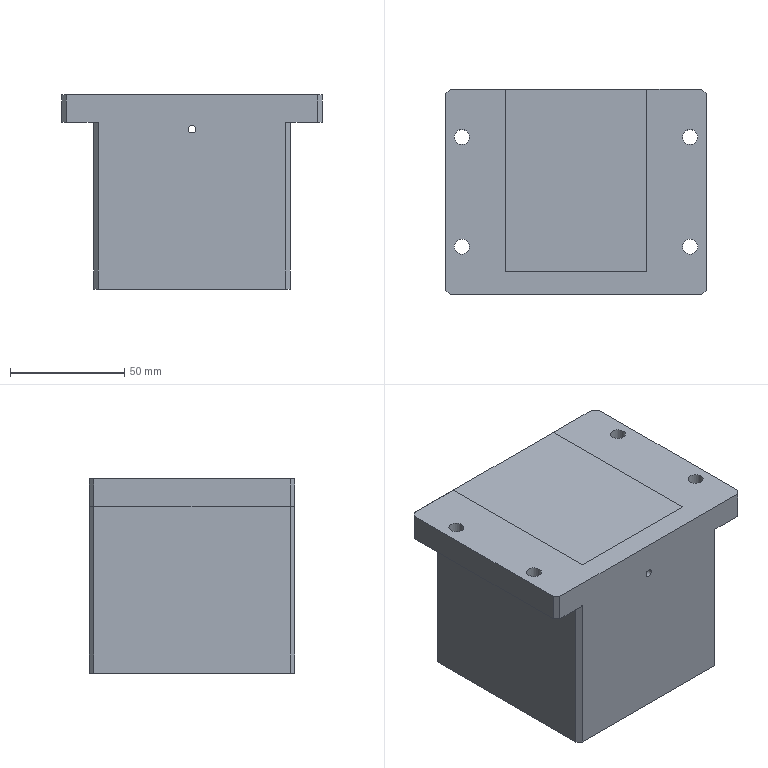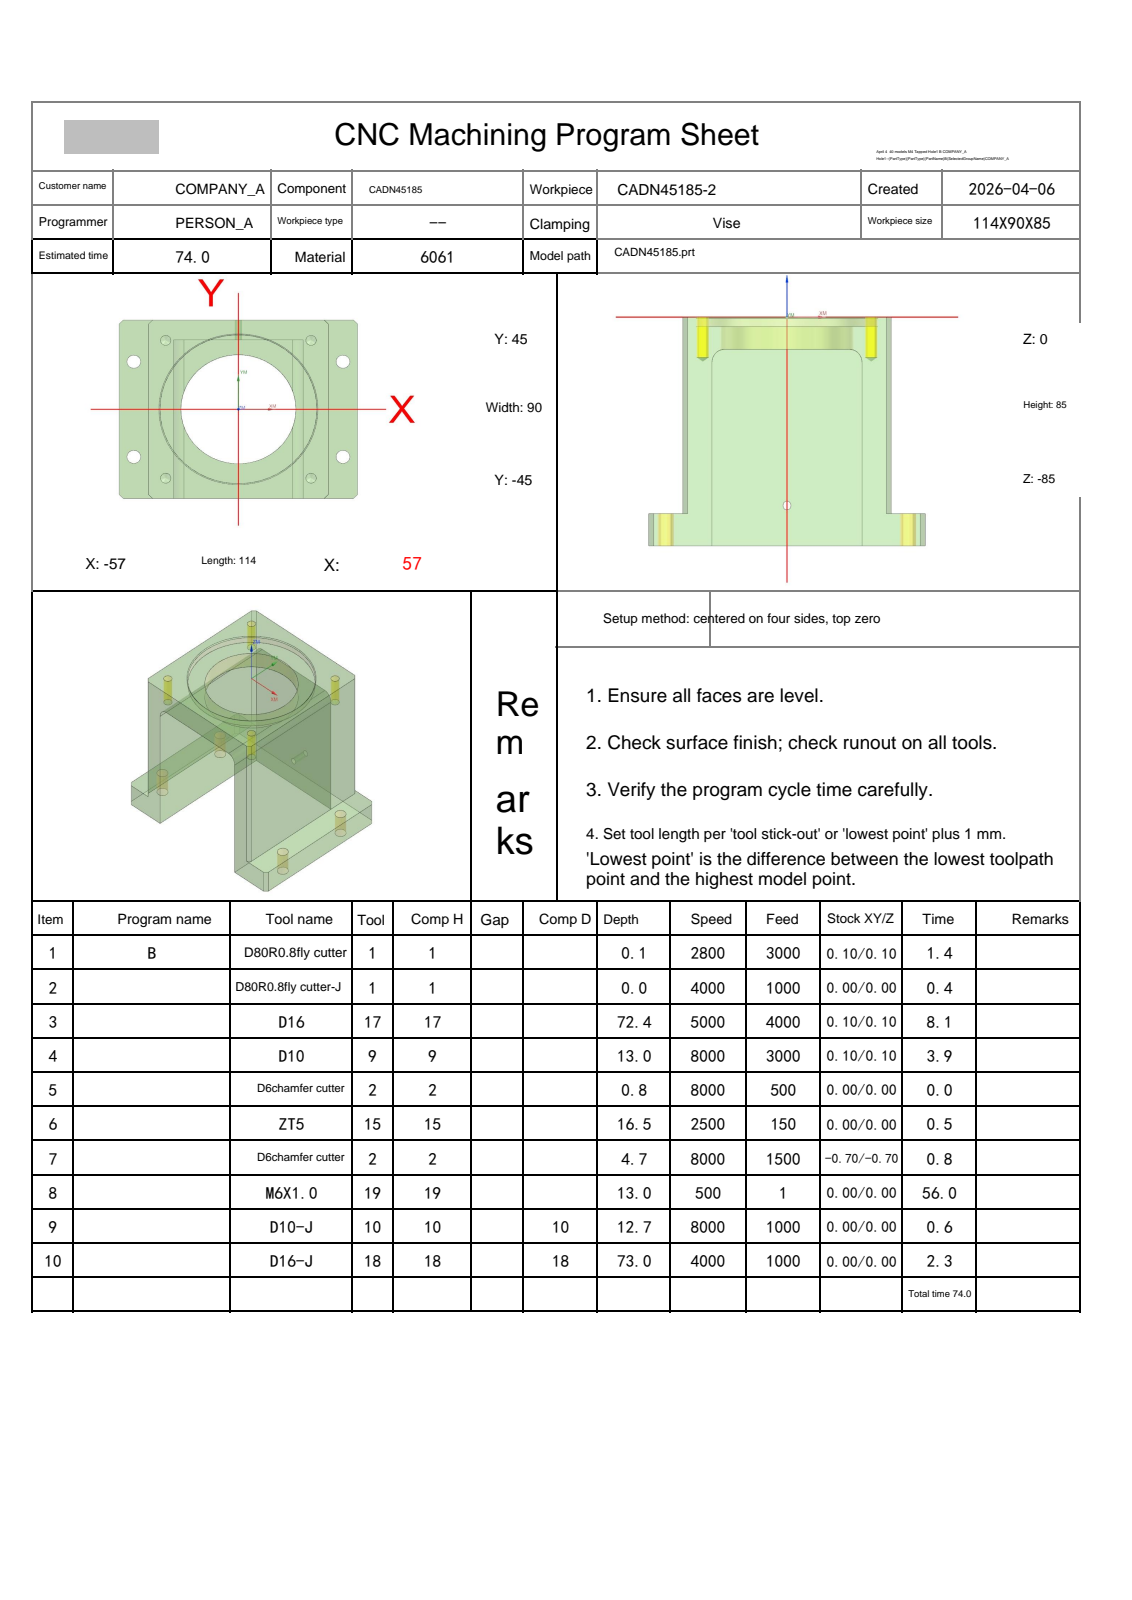NC program | NX | posted by the shop | part box 114 x 90 x 85 mm
Lines 1 to 2096 of 3620, first 1920 of 2094 lines:
%
O0001
(Machine time: 127.86 MIN)
(===Total Tool:8===)
(T1=D80R0.8飞刀 D=80.  R=0.8  D-  H01 Z=0.    )
(T17=D16    D=16.  R=0.   D-  H17 Z=-72.4 )
(T9=D10     D=10.  R=0.   D-  H09 Z=-13.  )
(T2=D6chamfer cutter   D=6.   R=0.   D-  H02 Z=-4.7  )
(T15=ZT5    D=5.   DR_a=118 D-  H15 Z=-16.5 )
(T19=M6X1.0 D=5.   DR_a=180 D-  H19 Z=-13.  )
(T10=D10-J  D=10.  R=0.   D10 H10 Z=-12.73)
(T18=D16-J  D=16.  R=0.   D18 H18 Z=-73.  )
G80 G90 G17 G49 G40
G91 G28 Z0
M01
N1 T01 M06
(D80R0.8飞刀  D=80. R=0.8 H=01 ce=0.10 di=0.10)
G00 G90 G54 X109.097 Y-21.097 M03 S2800
G43 H01 Z20.
M08
Z6.011
G01 Z4.011 F3000.
X97.097
X-89.897
G02 X-97.097 Y-13.897 I0.0 J7.2
G01 Y5.737
G02 X-89.097 Y13.737 I8. J0.0
G01 X97.097
X109.097
Z6.011
G00 Y-21.097
Z5.522
G01 Z3.522
X97.097
X-89.897
G02 X-97.097 Y-13.897 I0.0 J7.2
G01 Y5.737
G02 X-89.097 Y13.737 I8. J0.0
G01 X97.097
X109.097
Z5.522
G00 Y-21.097
Z5.033
G01 Z3.033
X97.097
X-89.897
G02 X-97.097 Y-13.897 I0.0 J7.2
G01 Y5.737
G02 X-89.097 Y13.737 I8. J0.0
G01 X97.097
X109.097
Z5.033
G00 Y-21.097
Z4.544
G01 Z2.544
X97.097
X-89.897
G02 X-97.097 Y-13.897 I0.0 J7.2
G01 Y5.737
G02 X-89.097 Y13.737 I8. J0.0
G01 X97.097
X109.097
Z4.544
G00 Y-21.097
Z4.056
G01 Z2.056
X97.097
X-89.897
G02 X-97.097 Y-13.897 I0.0 J7.2
G01 Y5.737
G02 X-89.097 Y13.737 I8. J0.0
G01 X97.097
X109.097
Z4.056
G00 Y-21.097
Z3.567
G01 Z1.567
X97.097
X-89.897
G02 X-97.097 Y-13.897 I0.0 J7.2
G01 Y5.737
G02 X-89.097 Y13.737 I8. J0.0
G01 X97.097
X109.097
Z3.567
G00 Y-21.097
Z3.078
G01 Z1.078
X97.097
X-89.897
G02 X-97.097 Y-13.897 I0.0 J7.2
G01 Y5.737
G02 X-89.097 Y13.737 I8. J0.0
G01 X97.097
X109.097
Z3.078
G00 Y-21.097
Z2.589
G01 Z.589
X97.097
X-89.897
G02 X-97.097 Y-13.897 I0.0 J7.2
G01 Y5.737
G02 X-89.097 Y13.737 I8. J0.0
G01 X97.097
X109.097
Z2.589
G00 Y-21.097
Z2.1
G01 Z.1
X97.097
X-89.897
G02 X-97.097 Y-13.897 I0.0 J7.2
G01 Y5.737
G02 X-89.097 Y13.737 I8. J0.0
G01 X97.097
X109.097
Z2.1
G00 Z20.
G91 G28 Z0.0
M05
M09
G91 G28 Z0.0
M01
N2 T01 M06
(D80R0.8飞刀-J  D=80. R=0.8 H=01 ce=0.00 di=0.00)
G00 G90 G54 X108.999 Y-20.999 M03 S4000
G43 H01 Z20.
M08
Z2.
G01 Z0.0 F1000.
X96.999
X-89.799
G02 X-96.999 Y-13.799 I0.0 J7.2
G01 Y5.639
G02 X-88.999 Y13.639 I8. J0.0
G01 X96.999
X108.999
Z2.
G00 Z20.
G91 G28 Z0.0
M05
M09
G91 G28 Z0.0
M01
N3 T17 M06
(D16  D=16. R=0. H=17 ce=0.10 di=0.10)
G00 G90 G54 X36.355 Y61.1 M03 S5000
G43 H17 Z20.
M08
Z-.598
G01 X46.728 Y50.728 F4000.
X48.728 Y48.728
G02 X51.1 Y43. I-5.728 J-5.728
G01 Y-43.
G02 X48.728 Y-48.728 I-8.1 J0.0
G01 X46.728 Y-50.728
X36.355 Y-61.1
G00 Z-1.197
G01 X46.728 Y-50.728
X48.728 Y-48.728
G03 X51.1 Y-43. I-5.728 J5.728
G01 Y43.
G03 X48.728 Y48.728 I-8.1 J0.0
G01 X46.728 Y50.728
X36.355 Y61.1
G00 Z-1.795
G01 X46.728 Y50.728
X48.728 Y48.728
G02 X51.1 Y43. I-5.728 J-5.728
G01 Y-43.
G02 X48.728 Y-48.728 I-8.1 J0.0
G01 X46.728 Y-50.728
X36.355 Y-61.1
G00 Z-2.393
G01 X46.728 Y-50.728
X48.728 Y-48.728
G03 X51.1 Y-43. I-5.728 J5.728
G01 Y43.
G03 X48.728 Y48.728 I-8.1 J0.0
G01 X46.728 Y50.728
X36.355 Y61.1
G00 Z-2.992
G01 X46.728 Y50.728
X48.728 Y48.728
G02 X51.1 Y43. I-5.728 J-5.728
G01 Y-43.
G02 X48.728 Y-48.728 I-8.1 J0.0
G01 X46.728 Y-50.728
X36.355 Y-61.1
G00 Z-3.59
G01 X46.728 Y-50.728
X48.728 Y-48.728
G03 X51.1 Y-43. I-5.728 J5.728
G01 Y43.
G03 X48.728 Y48.728 I-8.1 J0.0
G01 X46.728 Y50.728
X36.355 Y61.1
G00 Z-4.189
G01 X46.728 Y50.728
X48.728 Y48.728
G02 X51.1 Y43. I-5.728 J-5.728
G01 Y-43.
G02 X48.728 Y-48.728 I-8.1 J0.0
G01 X46.728 Y-50.728
X36.355 Y-61.1
G00 Z-4.787
G01 X46.728 Y-50.728
X48.728 Y-48.728
G03 X51.1 Y-43. I-5.728 J5.728
G01 Y43.
G03 X48.728 Y48.728 I-8.1 J0.0
G01 X46.728 Y50.728
X36.355 Y61.1
G00 Z-5.385
G01 X46.728 Y50.728
X48.728 Y48.728
G02 X51.1 Y43. I-5.728 J-5.728
G01 Y-43.
G02 X48.728 Y-48.728 I-8.1 J0.0
G01 X46.728 Y-50.728
X36.355 Y-61.1
G00 Z-5.984
G01 X46.728 Y-50.728
X48.728 Y-48.728
G03 X51.1 Y-43. I-5.728 J5.728
G01 Y43.
G03 X48.728 Y48.728 I-8.1 J0.0
G01 X46.728 Y50.728
X36.355 Y61.1
G00 Z-6.582
G01 X46.728 Y50.728
X48.728 Y48.728
G02 X51.1 Y43. I-5.728 J-5.728
G01 Y-43.
G02 X48.728 Y-48.728 I-8.1 J0.0
G01 X46.728 Y-50.728
X36.355 Y-61.1
G00 Z-7.18
G01 X46.728 Y-50.728
X48.728 Y-48.728
G03 X51.1 Y-43. I-5.728 J5.728
G01 Y43.
G03 X48.728 Y48.728 I-8.1 J0.0
G01 X46.728 Y50.728
X36.355 Y61.1
G00 Z-7.779
G01 X46.728 Y50.728
X48.728 Y48.728
G02 X51.1 Y43. I-5.728 J-5.728
G01 Y-43.
G02 X48.728 Y-48.728 I-8.1 J0.0
G01 X46.728 Y-50.728
X36.355 Y-61.1
G00 Z-8.377
G01 X46.728 Y-50.728
X48.728 Y-48.728
G03 X51.1 Y-43. I-5.728 J5.728
G01 Y43.
G03 X48.728 Y48.728 I-8.1 J0.0
G01 X46.728 Y50.728
X36.355 Y61.1
G00 Z-8.975
G01 X46.728 Y50.728
X48.728 Y48.728
G02 X51.1 Y43. I-5.728 J-5.728
G01 Y-43.
G02 X48.728 Y-48.728 I-8.1 J0.0
G01 X46.728 Y-50.728
X36.355 Y-61.1
G00 Z-9.574
G01 X46.728 Y-50.728
X48.728 Y-48.728
G03 X51.1 Y-43. I-5.728 J5.728
G01 Y43.
G03 X48.728 Y48.728 I-8.1 J0.0
G01 X46.728 Y50.728
X36.355 Y61.1
G00 Z-10.172
G01 X46.728 Y50.728
X48.728 Y48.728
G02 X51.1 Y43. I-5.728 J-5.728
G01 Y-43.
G02 X48.728 Y-48.728 I-8.1 J0.0
G01 X46.728 Y-50.728
X36.355 Y-61.1
G00 Z-10.77
G01 X46.728 Y-50.728
X48.728 Y-48.728
G03 X51.1 Y-43. I-5.728 J5.728
G01 Y43.
G03 X48.728 Y48.728 I-8.1 J0.0
G01 X46.728 Y50.728
X36.355 Y61.1
G00 Z-11.369
G01 X46.728 Y50.728
X48.728 Y48.728
G02 X51.1 Y43. I-5.728 J-5.728
G01 Y-43.
G02 X48.728 Y-48.728 I-8.1 J0.0
G01 X46.728 Y-50.728
X36.355 Y-61.1
G00 Z-11.967
G01 X46.728 Y-50.728
X48.728 Y-48.728
G03 X51.1 Y-43. I-5.728 J5.728
G01 Y43.
G03 X48.728 Y48.728 I-8.1 J0.0
G01 X46.728 Y50.728
X36.355 Y61.1
G00 Z-12.566
G01 X46.728 Y50.728
X48.728 Y48.728
G02 X51.1 Y43. I-5.728 J-5.728
G01 Y-43.
G02 X48.728 Y-48.728 I-8.1 J0.0
G01 X46.728 Y-50.728
X36.355 Y-61.1
G00 Z-13.164
G01 X46.728 Y-50.728
X48.728 Y-48.728
G03 X51.1 Y-43. I-5.728 J5.728
G01 Y43.
G03 X48.728 Y48.728 I-8.1 J0.0
G01 X46.728 Y50.728
X36.355 Y61.1
G00 Z-13.762
G01 X46.728 Y50.728
X48.728 Y48.728
G02 X51.1 Y43. I-5.728 J-5.728
G01 Y-43.
G02 X48.728 Y-48.728 I-8.1 J0.0
G01 X46.728 Y-50.728
X36.355 Y-61.1
G00 Z-14.361
G01 X46.728 Y-50.728
X48.728 Y-48.728
G03 X51.1 Y-43. I-5.728 J5.728
G01 Y43.
G03 X48.728 Y48.728 I-8.1 J0.0
G01 X46.728 Y50.728
X36.355 Y61.1
G00 Z-14.959
G01 X46.728 Y50.728
X48.728 Y48.728
G02 X51.1 Y43. I-5.728 J-5.728
G01 Y-43.
G02 X48.728 Y-48.728 I-8.1 J0.0
G01 X46.728 Y-50.728
X36.355 Y-61.1
G00 Z-15.557
G01 X46.728 Y-50.728
X48.728 Y-48.728
G03 X51.1 Y-43. I-5.728 J5.728
G01 Y43.
G03 X48.728 Y48.728 I-8.1 J0.0
G01 X46.728 Y50.728
X36.355 Y61.1
G00 Z-16.156
G01 X46.728 Y50.728
X48.728 Y48.728
G02 X51.1 Y43. I-5.728 J-5.728
G01 Y-43.
G02 X48.728 Y-48.728 I-8.1 J0.0
G01 X46.728 Y-50.728
X36.355 Y-61.1
G00 Z-16.754
G01 X46.728 Y-50.728
X48.728 Y-48.728
G03 X51.1 Y-43. I-5.728 J5.728
G01 Y43.
G03 X48.728 Y48.728 I-8.1 J0.0
G01 X46.728 Y50.728
X36.355 Y61.1
G00 Z-17.352
G01 X46.728 Y50.728
X48.728 Y48.728
G02 X51.1 Y43. I-5.728 J-5.728
G01 Y-43.
G02 X48.728 Y-48.728 I-8.1 J0.0
G01 X46.728 Y-50.728
X36.355 Y-61.1
G00 Z-17.951
G01 X46.728 Y-50.728
X48.728 Y-48.728
G03 X51.1 Y-43. I-5.728 J5.728
G01 Y43.
G03 X48.728 Y48.728 I-8.1 J0.0
G01 X46.728 Y50.728
X36.355 Y61.1
G00 Z-18.549
G01 X46.728 Y50.728
X48.728 Y48.728
G02 X51.1 Y43. I-5.728 J-5.728
G01 Y-43.
G02 X48.728 Y-48.728 I-8.1 J0.0
G01 X46.728 Y-50.728
X36.355 Y-61.1
G00 Z-19.148
G01 X46.728 Y-50.728
X48.728 Y-48.728
G03 X51.1 Y-43. I-5.728 J5.728
G01 Y43.
G03 X48.728 Y48.728 I-8.1 J0.0
G01 X46.728 Y50.728
X36.355 Y61.1
G00 Z-19.746
G01 X46.728 Y50.728
X48.728 Y48.728
G02 X51.1 Y43. I-5.728 J-5.728
G01 Y-43.
G02 X48.728 Y-48.728 I-8.1 J0.0
G01 X46.728 Y-50.728
X36.355 Y-61.1
G00 Z-20.344
G01 X46.728 Y-50.728
X48.728 Y-48.728
G03 X51.1 Y-43. I-5.728 J5.728
G01 Y43.
G03 X48.728 Y48.728 I-8.1 J0.0
G01 X46.728 Y50.728
X36.355 Y61.1
G00 Z-20.943
G01 X46.728 Y50.728
X48.728 Y48.728
G02 X51.1 Y43. I-5.728 J-5.728
G01 Y-43.
G02 X48.728 Y-48.728 I-8.1 J0.0
G01 X46.728 Y-50.728
X36.355 Y-61.1
G00 Z-21.541
G01 X46.728 Y-50.728
X48.728 Y-48.728
G03 X51.1 Y-43. I-5.728 J5.728
G01 Y43.
G03 X48.728 Y48.728 I-8.1 J0.0
G01 X46.728 Y50.728
X36.355 Y61.1
G00 Z-22.139
G01 X46.728 Y50.728
X48.728 Y48.728
G02 X51.1 Y43. I-5.728 J-5.728
G01 Y-43.
G02 X48.728 Y-48.728 I-8.1 J0.0
G01 X46.728 Y-50.728
X36.355 Y-61.1
G00 Z-22.738
G01 X46.728 Y-50.728
X48.728 Y-48.728
G03 X51.1 Y-43. I-5.728 J5.728
G01 Y43.
G03 X48.728 Y48.728 I-8.1 J0.0
G01 X46.728 Y50.728
X36.355 Y61.1
G00 Z-23.336
G01 X46.728 Y50.728
X48.728 Y48.728
G02 X51.1 Y43. I-5.728 J-5.728
G01 Y-43.
G02 X48.728 Y-48.728 I-8.1 J0.0
G01 X46.728 Y-50.728
X36.355 Y-61.1
G00 Z-23.934
G01 X46.728 Y-50.728
X48.728 Y-48.728
G03 X51.1 Y-43. I-5.728 J5.728
G01 Y43.
G03 X48.728 Y48.728 I-8.1 J0.0
G01 X46.728 Y50.728
X36.355 Y61.1
G00 Z-24.533
G01 X46.728 Y50.728
X48.728 Y48.728
G02 X51.1 Y43. I-5.728 J-5.728
G01 Y-43.
G02 X48.728 Y-48.728 I-8.1 J0.0
G01 X46.728 Y-50.728
X36.355 Y-61.1
G00 Z-25.131
G01 X46.728 Y-50.728
X48.728 Y-48.728
G03 X51.1 Y-43. I-5.728 J5.728
G01 Y43.
G03 X48.728 Y48.728 I-8.1 J0.0
G01 X46.728 Y50.728
X36.355 Y61.1
G00 Z-25.73
G01 X46.728 Y50.728
X48.728 Y48.728
G02 X51.1 Y43. I-5.728 J-5.728
G01 Y-43.
G02 X48.728 Y-48.728 I-8.1 J0.0
G01 X46.728 Y-50.728
X36.355 Y-61.1
G00 Z-26.328
G01 X46.728 Y-50.728
X48.728 Y-48.728
G03 X51.1 Y-43. I-5.728 J5.728
G01 Y43.
G03 X48.728 Y48.728 I-8.1 J0.0
G01 X46.728 Y50.728
X36.355 Y61.1
G00 Z-26.926
G01 X46.728 Y50.728
X48.728 Y48.728
G02 X51.1 Y43. I-5.728 J-5.728
G01 Y-43.
G02 X48.728 Y-48.728 I-8.1 J0.0
G01 X46.728 Y-50.728
X36.355 Y-61.1
G00 Z-27.525
G01 X46.728 Y-50.728
X48.728 Y-48.728
G03 X51.1 Y-43. I-5.728 J5.728
G01 Y43.
G03 X48.728 Y48.728 I-8.1 J0.0
G01 X46.728 Y50.728
X36.355 Y61.1
G00 Z-28.123
G01 X46.728 Y50.728
X48.728 Y48.728
G02 X51.1 Y43. I-5.728 J-5.728
G01 Y-43.
G02 X48.728 Y-48.728 I-8.1 J0.0
G01 X46.728 Y-50.728
X36.355 Y-61.1
G00 Z-28.721
G01 X46.728 Y-50.728
X48.728 Y-48.728
G03 X51.1 Y-43. I-5.728 J5.728
G01 Y43.
G03 X48.728 Y48.728 I-8.1 J0.0
G01 X46.728 Y50.728
X36.355 Y61.1
G00 Z-29.32
G01 X46.728 Y50.728
X48.728 Y48.728
G02 X51.1 Y43. I-5.728 J-5.728
G01 Y-43.
G02 X48.728 Y-48.728 I-8.1 J0.0
G01 X46.728 Y-50.728
X36.355 Y-61.1
G00 Z-29.918
G01 X46.728 Y-50.728
X48.728 Y-48.728
G03 X51.1 Y-43. I-5.728 J5.728
G01 Y43.
G03 X48.728 Y48.728 I-8.1 J0.0
G01 X46.728 Y50.728
X36.355 Y61.1
G00 Z-30.516
G01 X46.728 Y50.728
X48.728 Y48.728
G02 X51.1 Y43. I-5.728 J-5.728
G01 Y-43.
G02 X48.728 Y-48.728 I-8.1 J0.0
G01 X46.728 Y-50.728
X36.355 Y-61.1
G00 Z-31.115
G01 X46.728 Y-50.728
X48.728 Y-48.728
G03 X51.1 Y-43. I-5.728 J5.728
G01 Y43.
G03 X48.728 Y48.728 I-8.1 J0.0
G01 X46.728 Y50.728
X36.355 Y61.1
G00 Z-31.713
G01 X46.728 Y50.728
X48.728 Y48.728
G02 X51.1 Y43. I-5.728 J-5.728
G01 Y-43.
G02 X48.728 Y-48.728 I-8.1 J0.0
G01 X46.728 Y-50.728
X36.355 Y-61.1
G00 Z-32.311
G01 X46.728 Y-50.728
X48.728 Y-48.728
G03 X51.1 Y-43. I-5.728 J5.728
G01 Y43.
G03 X48.728 Y48.728 I-8.1 J0.0
G01 X46.728 Y50.728
X36.355 Y61.1
G00 Z-32.91
G01 X46.728 Y50.728
X48.728 Y48.728
G02 X51.1 Y43. I-5.728 J-5.728
G01 Y-43.
G02 X48.728 Y-48.728 I-8.1 J0.0
G01 X46.728 Y-50.728
X36.355 Y-61.1
G00 Z-33.508
G01 X46.728 Y-50.728
X48.728 Y-48.728
G03 X51.1 Y-43. I-5.728 J5.728
G01 Y43.
G03 X48.728 Y48.728 I-8.1 J0.0
G01 X46.728 Y50.728
X36.355 Y61.1
G00 Z-34.107
G01 X46.728 Y50.728
X48.728 Y48.728
G02 X51.1 Y43. I-5.728 J-5.728
G01 Y-43.
G02 X48.728 Y-48.728 I-8.1 J0.0
G01 X46.728 Y-50.728
X36.355 Y-61.1
G00 Z-34.705
G01 X46.728 Y-50.728
X48.728 Y-48.728
G03 X51.1 Y-43. I-5.728 J5.728
G01 Y43.
G03 X48.728 Y48.728 I-8.1 J0.0
G01 X46.728 Y50.728
X36.355 Y61.1
G00 Z-35.303
G01 X46.728 Y50.728
X48.728 Y48.728
G02 X51.1 Y43. I-5.728 J-5.728
G01 Y-43.
G02 X48.728 Y-48.728 I-8.1 J0.0
G01 X46.728 Y-50.728
X36.355 Y-61.1
G00 Z-35.902
G01 X46.728 Y-50.728
X48.728 Y-48.728
G03 X51.1 Y-43. I-5.728 J5.728
G01 Y43.
G03 X48.728 Y48.728 I-8.1 J0.0
G01 X46.728 Y50.728
X36.355 Y61.1
G00 Z-36.5
G01 X46.728 Y50.728
X48.728 Y48.728
G02 X51.1 Y43. I-5.728 J-5.728
G01 Y-43.
G02 X48.728 Y-48.728 I-8.1 J0.0
G01 X46.728 Y-50.728
X36.355 Y-61.1
G00 Z-37.098
G01 X46.728 Y-50.728
X48.728 Y-48.728
G03 X51.1 Y-43. I-5.728 J5.728
G01 Y43.
G03 X48.728 Y48.728 I-8.1 J0.0
G01 X46.728 Y50.728
X36.355 Y61.1
G00 Z-37.697
G01 X46.728 Y50.728
X48.728 Y48.728
G02 X51.1 Y43. I-5.728 J-5.728
G01 Y-43.
G02 X48.728 Y-48.728 I-8.1 J0.0
G01 X46.728 Y-50.728
X36.355 Y-61.1
G00 Z-38.295
G01 X46.728 Y-50.728
X48.728 Y-48.728
G03 X51.1 Y-43. I-5.728 J5.728
G01 Y43.
G03 X48.728 Y48.728 I-8.1 J0.0
G01 X46.728 Y50.728
X36.355 Y61.1
G00 Z-38.893
G01 X46.728 Y50.728
X48.728 Y48.728
G02 X51.1 Y43. I-5.728 J-5.728
G01 Y-43.
G02 X48.728 Y-48.728 I-8.1 J0.0
G01 X46.728 Y-50.728
X36.355 Y-61.1
G00 Z-39.492
G01 X46.728 Y-50.728
X48.728 Y-48.728
G03 X51.1 Y-43. I-5.728 J5.728
G01 Y43.
G03 X48.728 Y48.728 I-8.1 J0.0
G01 X46.728 Y50.728
X36.355 Y61.1
G00 Z-40.09
G01 X46.728 Y50.728
X48.728 Y48.728
G02 X51.1 Y43. I-5.728 J-5.728
G01 Y-43.
G02 X48.728 Y-48.728 I-8.1 J0.0
G01 X46.728 Y-50.728
X36.355 Y-61.1
G00 Z-40.689
G01 X46.728 Y-50.728
X48.728 Y-48.728
G03 X51.1 Y-43. I-5.728 J5.728
G01 Y43.
G03 X48.728 Y48.728 I-8.1 J0.0
G01 X46.728 Y50.728
X36.355 Y61.1
G00 Z-41.287
G01 X46.728 Y50.728
X48.728 Y48.728
G02 X51.1 Y43. I-5.728 J-5.728
G01 Y-43.
G02 X48.728 Y-48.728 I-8.1 J0.0
G01 X46.728 Y-50.728
X36.355 Y-61.1
G00 Z-41.885
G01 X46.728 Y-50.728
X48.728 Y-48.728
G03 X51.1 Y-43. I-5.728 J5.728
G01 Y43.
G03 X48.728 Y48.728 I-8.1 J0.0
G01 X46.728 Y50.728
X36.355 Y61.1
G00 Z-42.484
G01 X46.728 Y50.728
X48.728 Y48.728
G02 X51.1 Y43. I-5.728 J-5.728
G01 Y-43.
G02 X48.728 Y-48.728 I-8.1 J0.0
G01 X46.728 Y-50.728
X36.355 Y-61.1
G00 Z-43.082
G01 X46.728 Y-50.728
X48.728 Y-48.728
G03 X51.1 Y-43. I-5.728 J5.728
G01 Y43.
G03 X48.728 Y48.728 I-8.1 J0.0
G01 X46.728 Y50.728
X36.355 Y61.1
G00 Z-43.68
G01 X46.728 Y50.728
X48.728 Y48.728
G02 X51.1 Y43. I-5.728 J-5.728
G01 Y-43.
G02 X48.728 Y-48.728 I-8.1 J0.0
G01 X46.728 Y-50.728
X36.355 Y-61.1
G00 Z-44.279
G01 X46.728 Y-50.728
X48.728 Y-48.728
G03 X51.1 Y-43. I-5.728 J5.728
G01 Y43.
G03 X48.728 Y48.728 I-8.1 J0.0
G01 X46.728 Y50.728
X36.355 Y61.1
G00 Z-44.877
G01 X46.728 Y50.728
X48.728 Y48.728
G02 X51.1 Y43. I-5.728 J-5.728
G01 Y-43.
G02 X48.728 Y-48.728 I-8.1 J0.0
G01 X46.728 Y-50.728
X36.355 Y-61.1
G00 Z-45.475
G01 X46.728 Y-50.728
X48.728 Y-48.728
G03 X51.1 Y-43. I-5.728 J5.728
G01 Y43.
G03 X48.728 Y48.728 I-8.1 J0.0
G01 X46.728 Y50.728
X36.355 Y61.1
G00 Z-46.074
G01 X46.728 Y50.728
X48.728 Y48.728
G02 X51.1 Y43. I-5.728 J-5.728
G01 Y-43.
G02 X48.728 Y-48.728 I-8.1 J0.0
G01 X46.728 Y-50.728
X36.355 Y-61.1
G00 Z-46.672
G01 X46.728 Y-50.728
X48.728 Y-48.728
G03 X51.1 Y-43. I-5.728 J5.728
G01 Y43.
G03 X48.728 Y48.728 I-8.1 J0.0
G01 X46.728 Y50.728
X36.355 Y61.1
G00 Z-47.27
G01 X46.728 Y50.728
X48.728 Y48.728
G02 X51.1 Y43. I-5.728 J-5.728
G01 Y-43.
G02 X48.728 Y-48.728 I-8.1 J0.0
G01 X46.728 Y-50.728
X36.355 Y-61.1
G00 Z-47.869
G01 X46.728 Y-50.728
X48.728 Y-48.728
G03 X51.1 Y-43. I-5.728 J5.728
G01 Y43.
G03 X48.728 Y48.728 I-8.1 J0.0
G01 X46.728 Y50.728
X36.355 Y61.1
G00 Z-48.467
G01 X46.728 Y50.728
X48.728 Y48.728
G02 X51.1 Y43. I-5.728 J-5.728
G01 Y-43.
G02 X48.728 Y-48.728 I-8.1 J0.0
G01 X46.728 Y-50.728
X36.355 Y-61.1
G00 Z-49.066
G01 X46.728 Y-50.728
X48.728 Y-48.728
G03 X51.1 Y-43. I-5.728 J5.728
G01 Y43.
G03 X48.728 Y48.728 I-8.1 J0.0
G01 X46.728 Y50.728
X36.355 Y61.1
G00 Z-49.664
G01 X46.728 Y50.728
X48.728 Y48.728
G02 X51.1 Y43. I-5.728 J-5.728
G01 Y-43.
G02 X48.728 Y-48.728 I-8.1 J0.0
G01 X46.728 Y-50.728
X36.355 Y-61.1
G00 Z-50.262
G01 X46.728 Y-50.728
X48.728 Y-48.728
G03 X51.1 Y-43. I-5.728 J5.728
G01 Y43.
G03 X48.728 Y48.728 I-8.1 J0.0
G01 X46.728 Y50.728
X36.355 Y61.1
G00 Z-50.861
G01 X46.728 Y50.728
X48.728 Y48.728
G02 X51.1 Y43. I-5.728 J-5.728
G01 Y-43.
G02 X48.728 Y-48.728 I-8.1 J0.0
G01 X46.728 Y-50.728
X36.355 Y-61.1
G00 Z-51.459
G01 X46.728 Y-50.728
X48.728 Y-48.728
G03 X51.1 Y-43. I-5.728 J5.728
G01 Y43.
G03 X48.728 Y48.728 I-8.1 J0.0
G01 X46.728 Y50.728
X36.355 Y61.1
G00 Z-52.057
G01 X46.728 Y50.728
X48.728 Y48.728
G02 X51.1 Y43. I-5.728 J-5.728
G01 Y-43.
G02 X48.728 Y-48.728 I-8.1 J0.0
G01 X46.728 Y-50.728
X36.355 Y-61.1
G00 Z-52.656
G01 X46.728 Y-50.728
X48.728 Y-48.728
G03 X51.1 Y-43. I-5.728 J5.728
G01 Y43.
G03 X48.728 Y48.728 I-8.1 J0.0
G01 X46.728 Y50.728
X36.355 Y61.1
G00 Z-53.254
G01 X46.728 Y50.728
X48.728 Y48.728
G02 X51.1 Y43. I-5.728 J-5.728
G01 Y-43.
G02 X48.728 Y-48.728 I-8.1 J0.0
G01 X46.728 Y-50.728
X36.355 Y-61.1
G00 Z-53.852
G01 X46.728 Y-50.728
X48.728 Y-48.728
G03 X51.1 Y-43. I-5.728 J5.728
G01 Y43.
G03 X48.728 Y48.728 I-8.1 J0.0
G01 X46.728 Y50.728
X36.355 Y61.1
G00 Z-54.451
G01 X46.728 Y50.728
X48.728 Y48.728
G02 X51.1 Y43. I-5.728 J-5.728
G01 Y-43.
G02 X48.728 Y-48.728 I-8.1 J0.0
G01 X46.728 Y-50.728
X36.355 Y-61.1
G00 Z-55.049
G01 X46.728 Y-50.728
X48.728 Y-48.728
G03 X51.1 Y-43. I-5.728 J5.728
G01 Y43.
G03 X48.728 Y48.728 I-8.1 J0.0
G01 X46.728 Y50.728
X36.355 Y61.1
G00 Z-55.648
G01 X46.728 Y50.728
X48.728 Y48.728
G02 X51.1 Y43. I-5.728 J-5.728
G01 Y-43.
G02 X48.728 Y-48.728 I-8.1 J0.0
G01 X46.728 Y-50.728
X36.355 Y-61.1
G00 Z-56.246
G01 X46.728 Y-50.728
X48.728 Y-48.728
G03 X51.1 Y-43. I-5.728 J5.728
G01 Y43.
G03 X48.728 Y48.728 I-8.1 J0.0
G01 X46.728 Y50.728
X36.355 Y61.1
G00 Z-56.844
G01 X46.728 Y50.728
X48.728 Y48.728
G02 X51.1 Y43. I-5.728 J-5.728
G01 Y-43.
G02 X48.728 Y-48.728 I-8.1 J0.0
G01 X46.728 Y-50.728
X36.355 Y-61.1
G00 Z-57.443
G01 X46.728 Y-50.728
X48.728 Y-48.728
G03 X51.1 Y-43. I-5.728 J5.728
G01 Y43.
G03 X48.728 Y48.728 I-8.1 J0.0
G01 X46.728 Y50.728
X36.355 Y61.1
G00 Z-58.041
G01 X46.728 Y50.728
X48.728 Y48.728
G02 X51.1 Y43. I-5.728 J-5.728
G01 Y-43.
G02 X48.728 Y-48.728 I-8.1 J0.0
G01 X46.728 Y-50.728
X36.355 Y-61.1
G00 Z-58.639
G01 X46.728 Y-50.728
X48.728 Y-48.728
G03 X51.1 Y-43. I-5.728 J5.728
G01 Y43.
G03 X48.728 Y48.728 I-8.1 J0.0
G01 X46.728 Y50.728
X36.355 Y61.1
G00 Z-59.238
G01 X46.728 Y50.728
X48.728 Y48.728
G02 X51.1 Y43. I-5.728 J-5.728
G01 Y-43.
G02 X48.728 Y-48.728 I-8.1 J0.0
G01 X46.728 Y-50.728
X36.355 Y-61.1
G00 Z-59.836
G01 X46.728 Y-50.728
X48.728 Y-48.728
G03 X51.1 Y-43. I-5.728 J5.728
G01 Y43.
G03 X48.728 Y48.728 I-8.1 J0.0
G01 X46.728 Y50.728
X36.355 Y61.1
G00 Z-60.434
G01 X46.728 Y50.728
X48.728 Y48.728
G02 X51.1 Y43. I-5.728 J-5.728
G01 Y-43.
G02 X48.728 Y-48.728 I-8.1 J0.0
G01 X46.728 Y-50.728
X36.355 Y-61.1
G00 Z-61.033
G01 X46.728 Y-50.728
X48.728 Y-48.728
G03 X51.1 Y-43. I-5.728 J5.728
G01 Y43.
G03 X48.728 Y48.728 I-8.1 J0.0
G01 X46.728 Y50.728
X36.355 Y61.1
G00 Z-61.631
G01 X46.728 Y50.728
X48.728 Y48.728
G02 X51.1 Y43. I-5.728 J-5.728
G01 Y-43.
G02 X48.728 Y-48.728 I-8.1 J0.0
G01 X46.728 Y-50.728
X36.355 Y-61.1
G00 Z-62.23
G01 X46.728 Y-50.728
X48.728 Y-48.728
G03 X51.1 Y-43. I-5.728 J5.728
G01 Y43.
G03 X48.728 Y48.728 I-8.1 J0.0
G01 X46.728 Y50.728
X36.355 Y61.1
G00 Z-62.828
G01 X46.728 Y50.728
X48.728 Y48.728
G02 X51.1 Y43. I-5.728 J-5.728
G01 Y-43.
G02 X48.728 Y-48.728 I-8.1 J0.0
G01 X46.728 Y-50.728
X36.355 Y-61.1
G00 Z-63.426
G01 X46.728 Y-50.728
X48.728 Y-48.728
G03 X51.1 Y-43. I-5.728 J5.728
G01 Y43.
G03 X48.728 Y48.728 I-8.1 J0.0
G01 X46.728 Y50.728
X36.355 Y61.1
G00 Z-64.025
G01 X46.728 Y50.728
X48.728 Y48.728
G02 X51.1 Y43. I-5.728 J-5.728
G01 Y-43.
G02 X48.728 Y-48.728 I-8.1 J0.0
G01 X46.728 Y-50.728
X36.355 Y-61.1
G00 Z-64.623
G01 X46.728 Y-50.728
X48.728 Y-48.728
G03 X51.1 Y-43. I-5.728 J5.728
G01 Y43.
G03 X48.728 Y48.728 I-8.1 J0.0
G01 X46.728 Y50.728
X36.355 Y61.1
G00 Z-65.221
G01 X46.728 Y50.728
X48.728 Y48.728
G02 X51.1 Y43. I-5.728 J-5.728
G01 Y-43.
G02 X48.728 Y-48.728 I-8.1 J0.0
G01 X46.728 Y-50.728
X36.355 Y-61.1
G00 Z-65.82
G01 X46.728 Y-50.728
X48.728 Y-48.728
G03 X51.1 Y-43. I-5.728 J5.728
G01 Y43.
G03 X48.728 Y48.728 I-8.1 J0.0
G01 X46.728 Y50.728
X36.355 Y61.1
G00 Z-66.418
G01 X46.728 Y50.728
X48.728 Y48.728
G02 X51.1 Y43. I-5.728 J-5.728
G01 Y-43.
G02 X48.728 Y-48.728 I-8.1 J0.0
G01 X46.728 Y-50.728
X36.355 Y-61.1
G00 Z-67.016
G01 X46.728 Y-50.728
X48.728 Y-48.728
G03 X51.1 Y-43. I-5.728 J5.728
G01 Y43.
G03 X48.728 Y48.728 I-8.1 J0.0
G01 X46.728 Y50.728
X36.355 Y61.1
G00 Z-67.615
G01 X46.728 Y50.728
X48.728 Y48.728
G02 X51.1 Y43. I-5.728 J-5.728
G01 Y-43.
G02 X48.728 Y-48.728 I-8.1 J0.0
G01 X46.728 Y-50.728
X36.355 Y-61.1
G00 Z-68.213
G01 X46.728 Y-50.728
X48.728 Y-48.728
G03 X51.1 Y-43. I-5.728 J5.728
G01 Y43.
G03 X48.728 Y48.728 I-8.1 J0.0
G01 X46.728 Y50.728
X36.355 Y61.1
G00 Z-68.811
G01 X46.728 Y50.728
X48.728 Y48.728
G02 X51.1 Y43. I-5.728 J-5.728
G01 Y-43.
G02 X48.728 Y-48.728 I-8.1 J0.0
G01 X46.728 Y-50.728
X36.355 Y-61.1
G00 Z-69.41
G01 X46.728 Y-50.728
X48.728 Y-48.728
G03 X51.1 Y-43. I-5.728 J5.728
G01 Y43.
G03 X48.728 Y48.728 I-8.1 J0.0
G01 X46.728 Y50.728
X36.355 Y61.1
G00 Z-70.008
G01 X46.728 Y50.728
X48.728 Y48.728
G02 X51.1 Y43. I-5.728 J-5.728
G01 Y-43.
G02 X48.728 Y-48.728 I-8.1 J0.0
G01 X46.728 Y-50.728
X36.355 Y-61.1
G00 Z-70.607
G01 X46.728 Y-50.728
X48.728 Y-48.728
G03 X51.1 Y-43. I-5.728 J5.728
G01 Y43.
G03 X48.728 Y48.728 I-8.1 J0.0
G01 X46.728 Y50.728
X36.355 Y61.1
G00 Z-71.205
G01 X46.728 Y50.728
X48.728 Y48.728
G02 X51.1 Y43. I-5.728 J-5.728
G01 Y-43.
G02 X48.728 Y-48.728 I-8.1 J0.0
G01 X46.728 Y-50.728
X36.355 Y-61.1
G00 Z-71.803
G01 X46.728 Y-50.728
X48.728 Y-48.728
G03 X51.1 Y-43. I-5.728 J5.728
G01 Y43.
G03 X48.728 Y48.728 I-8.1 J0.0
G01 X46.728 Y50.728
X36.355 Y61.1
G00 Z-72.402
G01 X46.728 Y50.728
X48.728 Y48.728
G02 X51.1 Y43. I-5.728 J-5.728
G01 Y-43.
G02 X48.728 Y-48.728 I-8.1 J0.0
G01 X46.728 Y-50.728
X36.355 Y-61.1
G00 Z20.
X-36.355
Z-.598
G01 X-46.728 Y-50.728
X-48.728 Y-48.728
G02 X-51.1 Y-43. I5.728 J5.728
G01 Y43.
G02 X-48.728 Y48.728 I8.1 J0.0
G01 X-46.728 Y50.728
X-36.355 Y61.1
G00 Z-1.197
G01 X-46.728 Y50.728
X-48.728 Y48.728
G03 X-51.1 Y43. I5.728 J-5.728
G01 Y-43.
G03 X-48.728 Y-48.728 I8.1 J0.0
G01 X-46.728 Y-50.728
X-36.355 Y-61.1
G00 Z-1.795
G01 X-46.728 Y-50.728
X-48.728 Y-48.728
G02 X-51.1 Y-43. I5.728 J5.728
G01 Y43.
G02 X-48.728 Y48.728 I8.1 J0.0
G01 X-46.728 Y50.728
X-36.355 Y61.1
G00 Z-2.393
G01 X-46.728 Y50.728
X-48.728 Y48.728
G03 X-51.1 Y43. I5.728 J-5.728
G01 Y-43.
G03 X-48.728 Y-48.728 I8.1 J0.0
G01 X-46.728 Y-50.728
X-36.355 Y-61.1
G00 Z-2.992
G01 X-46.728 Y-50.728
X-48.728 Y-48.728
G02 X-51.1 Y-43. I5.728 J5.728
G01 Y43.
G02 X-48.728 Y48.728 I8.1 J0.0
G01 X-46.728 Y50.728
X-36.355 Y61.1
G00 Z-3.59
G01 X-46.728 Y50.728
X-48.728 Y48.728
G03 X-51.1 Y43. I5.728 J-5.728
G01 Y-43.
G03 X-48.728 Y-48.728 I8.1 J0.0
G01 X-46.728 Y-50.728
X-36.355 Y-61.1
G00 Z-4.189
G01 X-46.728 Y-50.728
X-48.728 Y-48.728
G02 X-51.1 Y-43. I5.728 J5.728
G01 Y43.
G02 X-48.728 Y48.728 I8.1 J0.0
G01 X-46.728 Y50.728
X-36.355 Y61.1
G00 Z-4.787
G01 X-46.728 Y50.728
X-48.728 Y48.728
G03 X-51.1 Y43. I5.728 J-5.728
G01 Y-43.
G03 X-48.728 Y-48.728 I8.1 J0.0
G01 X-46.728 Y-50.728
X-36.355 Y-61.1
G00 Z-5.385
G01 X-46.728 Y-50.728
X-48.728 Y-48.728
G02 X-51.1 Y-43. I5.728 J5.728
G01 Y43.
G02 X-48.728 Y48.728 I8.1 J0.0
G01 X-46.728 Y50.728
X-36.355 Y61.1
G00 Z-5.984
G01 X-46.728 Y50.728
X-48.728 Y48.728
G03 X-51.1 Y43. I5.728 J-5.728
G01 Y-43.
G03 X-48.728 Y-48.728 I8.1 J0.0
G01 X-46.728 Y-50.728
X-36.355 Y-61.1
G00 Z-6.582
G01 X-46.728 Y-50.728
X-48.728 Y-48.728
G02 X-51.1 Y-43. I5.728 J5.728
G01 Y43.
G02 X-48.728 Y48.728 I8.1 J0.0
G01 X-46.728 Y50.728
X-36.355 Y61.1
G00 Z-7.18
G01 X-46.728 Y50.728
X-48.728 Y48.728
G03 X-51.1 Y43. I5.728 J-5.728
G01 Y-43.
G03 X-48.728 Y-48.728 I8.1 J0.0
G01 X-46.728 Y-50.728
X-36.355 Y-61.1
G00 Z-7.779
G01 X-46.728 Y-50.728
X-48.728 Y-48.728
G02 X-51.1 Y-43. I5.728 J5.728
G01 Y43.
G02 X-48.728 Y48.728 I8.1 J0.0
G01 X-46.728 Y50.728
X-36.355 Y61.1
G00 Z-8.377
G01 X-46.728 Y50.728
X-48.728 Y48.728
G03 X-51.1 Y43. I5.728 J-5.728
G01 Y-43.
G03 X-48.728 Y-48.728 I8.1 J0.0
G01 X-46.728 Y-50.728
X-36.355 Y-61.1
G00 Z-8.975
G01 X-46.728 Y-50.728
X-48.728 Y-48.728
G02 X-51.1 Y-43. I5.728 J5.728
G01 Y43.
G02 X-48.728 Y48.728 I8.1 J0.0
G01 X-46.728 Y50.728
X-36.355 Y61.1
G00 Z-9.574
G01 X-46.728 Y50.728
X-48.728 Y48.728
G03 X-51.1 Y43. I5.728 J-5.728
G01 Y-43.
G03 X-48.728 Y-48.728 I8.1 J0.0
G01 X-46.728 Y-50.728
X-36.355 Y-61.1
G00 Z-10.172
G01 X-46.728 Y-50.728
X-48.728 Y-48.728
G02 X-51.1 Y-43. I5.728 J5.728
G01 Y43.
G02 X-48.728 Y48.728 I8.1 J0.0
G01 X-46.728 Y50.728
X-36.355 Y61.1
G00 Z-10.77
G01 X-46.728 Y50.728
X-48.728 Y48.728
G03 X-51.1 Y43. I5.728 J-5.728
G01 Y-43.
G03 X-48.728 Y-48.728 I8.1 J0.0
G01 X-46.728 Y-50.728
X-36.355 Y-61.1
G00 Z-11.369
G01 X-46.728 Y-50.728
X-48.728 Y-48.728
G02 X-51.1 Y-43. I5.728 J5.728
G01 Y43.
G02 X-48.728 Y48.728 I8.1 J0.0
G01 X-46.728 Y50.728
X-36.355 Y61.1
G00 Z-11.967
G01 X-46.728 Y50.728
X-48.728 Y48.728
G03 X-51.1 Y43. I5.728 J-5.728
G01 Y-43.
G03 X-48.728 Y-48.728 I8.1 J0.0
G01 X-46.728 Y-50.728
X-36.355 Y-61.1
G00 Z-12.566
G01 X-46.728 Y-50.728
X-48.728 Y-48.728
G02 X-51.1 Y-43. I5.728 J5.728
G01 Y43.
G02 X-48.728 Y48.728 I8.1 J0.0
G01 X-46.728 Y50.728
X-36.355 Y61.1
G00 Z-13.164
G01 X-46.728 Y50.728
X-48.728 Y48.728
G03 X-51.1 Y43. I5.728 J-5.728
G01 Y-43.
G03 X-48.728 Y-48.728 I8.1 J0.0
G01 X-46.728 Y-50.728
X-36.355 Y-61.1
G00 Z-13.762
G01 X-46.728 Y-50.728
X-48.728 Y-48.728
G02 X-51.1 Y-43. I5.728 J5.728
G01 Y43.
G02 X-48.728 Y48.728 I8.1 J0.0
G01 X-46.728 Y50.728
X-36.355 Y61.1
G00 Z-14.361
G01 X-46.728 Y50.728
X-48.728 Y48.728
G03 X-51.1 Y43. I5.728 J-5.728
G01 Y-43.
G03 X-48.728 Y-48.728 I8.1 J0.0
G01 X-46.728 Y-50.728
X-36.355 Y-61.1
G00 Z-14.959
G01 X-46.728 Y-50.728
X-48.728 Y-48.728
G02 X-51.1 Y-43. I5.728 J5.728
G01 Y43.
G02 X-48.728 Y48.728 I8.1 J0.0
G01 X-46.728 Y50.728
X-36.355 Y61.1
G00 Z-15.557
G01 X-46.728 Y50.728
X-48.728 Y48.728
G03 X-51.1 Y43. I5.728 J-5.728
G01 Y-43.
G03 X-48.728 Y-48.728 I8.1 J0.0
G01 X-46.728 Y-50.728
X-36.355 Y-61.1
G00 Z-16.156
G01 X-46.728 Y-50.728
X-48.728 Y-48.728
G02 X-51.1 Y-43. I5.728 J5.728
G01 Y43.
G02 X-48.728 Y48.728 I8.1 J0.0
G01 X-46.728 Y50.728
X-36.355 Y61.1
G00 Z-16.754
G01 X-46.728 Y50.728
X-48.728 Y48.728
G03 X-51.1 Y43. I5.728 J-5.728
G01 Y-43.
G03 X-48.728 Y-48.728 I8.1 J0.0
G01 X-46.728 Y-50.728
X-36.355 Y-61.1
G00 Z-17.352
G01 X-46.728 Y-50.728
X-48.728 Y-48.728
G02 X-51.1 Y-43. I5.728 J5.728
G01 Y43.
G02 X-48.728 Y48.728 I8.1 J0.0
G01 X-46.728 Y50.728
X-36.355 Y61.1
G00 Z-17.951
G01 X-46.728 Y50.728
X-48.728 Y48.728
G03 X-51.1 Y43. I5.728 J-5.728
G01 Y-43.
G03 X-48.728 Y-48.728 I8.1 J0.0
G01 X-46.728 Y-50.728
X-36.355 Y-61.1
G00 Z-18.549
G01 X-46.728 Y-50.728
X-48.728 Y-48.728
G02 X-51.1 Y-43. I5.728 J5.728
G01 Y43.
G02 X-48.728 Y48.728 I8.1 J0.0
G01 X-46.728 Y50.728
X-36.355 Y61.1
G00 Z-19.148
G01 X-46.728 Y50.728
X-48.728 Y48.728
G03 X-51.1 Y43. I5.728 J-5.728
G01 Y-43.
G03 X-48.728 Y-48.728 I8.1 J0.0
G01 X-46.728 Y-50.728
X-36.355 Y-61.1
G00 Z-19.746
G01 X-46.728 Y-50.728
X-48.728 Y-48.728
G02 X-51.1 Y-43. I5.728 J5.728
G01 Y43.
G02 X-48.728 Y48.728 I8.1 J0.0
G01 X-46.728 Y50.728
X-36.355 Y61.1
G00 Z-20.344
G01 X-46.728 Y50.728
X-48.728 Y48.728
G03 X-51.1 Y43. I5.728 J-5.728
G01 Y-43.
G03 X-48.728 Y-48.728 I8.1 J0.0
G01 X-46.728 Y-50.728
X-36.355 Y-61.1
G00 Z-20.943
G01 X-46.728 Y-50.728
X-48.728 Y-48.728
G02 X-51.1 Y-43. I5.728 J5.728
G01 Y43.
G02 X-48.728 Y48.728 I8.1 J0.0
G01 X-46.728 Y50.728
X-36.355 Y61.1
G00 Z-21.541
G01 X-46.728 Y50.728
X-48.728 Y48.728
G03 X-51.1 Y43. I5.728 J-5.728
G01 Y-43.
G03 X-48.728 Y-48.728 I8.1 J0.0
G01 X-46.728 Y-50.728
X-36.355 Y-61.1
G00 Z-22.139
G01 X-46.728 Y-50.728
X-48.728 Y-48.728
G02 X-51.1 Y-43. I5.728 J5.728
G01 Y43.
G02 X-48.728 Y48.728 I8.1 J0.0
G01 X-46.728 Y50.728
X-36.355 Y61.1
G00 Z-22.738
G01 X-46.728 Y50.728
X-48.728 Y48.728
G03 X-51.1 Y43. I5.728 J-5.728
G01 Y-43.
G03 X-48.728 Y-48.728 I8.1 J0.0
G01 X-46.728 Y-50.728
X-36.355 Y-61.1
G00 Z-23.336
G01 X-46.728 Y-50.728
X-48.728 Y-48.728
G02 X-51.1 Y-43. I5.728 J5.728
G01 Y43.
G02 X-48.728 Y48.728 I8.1 J0.0
G01 X-46.728 Y50.728
X-36.355 Y61.1
G00 Z-23.934
G01 X-46.728 Y50.728
X-48.728 Y48.728
G03 X-51.1 Y43. I5.728 J-5.728
G01 Y-43.
G03 X-48.728 Y-48.728 I8.1 J0.0
G01 X-46.728 Y-50.728
X-36.355 Y-61.1
G00 Z-24.533
G01 X-46.728 Y-50.728
X-48.728 Y-48.728
G02 X-51.1 Y-43. I5.728 J5.728
G01 Y43.
G02 X-48.728 Y48.728 I8.1 J0.0
G01 X-46.728 Y50.728
X-36.355 Y61.1
G00 Z-25.131
G01 X-46.728 Y50.728
X-48.728 Y48.728
G03 X-51.1 Y43. I5.728 J-5.728
G01 Y-43.
G03 X-48.728 Y-48.728 I8.1 J0.0
G01 X-46.728 Y-50.728
X-36.355 Y-61.1
G00 Z-25.73
G01 X-46.728 Y-50.728
X-48.728 Y-48.728
G02 X-51.1 Y-43. I5.728 J5.728
G01 Y43.
G02 X-48.728 Y48.728 I8.1 J0.0
G01 X-46.728 Y50.728
X-36.355 Y61.1
G00 Z-26.328
G01 X-46.728 Y50.728
X-48.728 Y48.728
G03 X-51.1 Y43. I5.728 J-5.728
G01 Y-43.
G03 X-48.728 Y-48.728 I8.1 J0.0
G01 X-46.728 Y-50.728
X-36.355 Y-61.1
G00 Z-26.926
G01 X-46.728 Y-50.728
X-48.728 Y-48.728
G02 X-51.1 Y-43. I5.728 J5.728
G01 Y43.
G02 X-48.728 Y48.728 I8.1 J0.0
G01 X-46.728 Y50.728
X-36.355 Y61.1
G00 Z-27.525
G01 X-46.728 Y50.728
X-48.728 Y48.728
G03 X-51.1 Y43. I5.728 J-5.728
G01 Y-43.
G03 X-48.728 Y-48.728 I8.1 J0.0
G01 X-46.728 Y-50.728
X-36.355 Y-61.1
G00 Z-28.123
G01 X-46.728 Y-50.728
X-48.728 Y-48.728
G02 X-51.1 Y-43. I5.728 J5.728
G01 Y43.
G02 X-48.728 Y48.728 I8.1 J0.0
G01 X-46.728 Y50.728
X-36.355 Y61.1
G00 Z-28.721
G01 X-46.728 Y50.728
X-48.728 Y48.728
G03 X-51.1 Y43. I5.728 J-5.728
G01 Y-43.
G03 X-48.728 Y-48.728 I8.1 J0.0
G01 X-46.728 Y-50.728
X-36.355 Y-61.1
G00 Z-29.32
G01 X-46.728 Y-50.728
X-48.728 Y-48.728
G02 X-51.1 Y-43. I5.728 J5.728
G01 Y43.
G02 X-48.728 Y48.728 I8.1 J0.0
G01 X-46.728 Y50.728
X-36.355 Y61.1
G00 Z-29.918
G01 X-46.728 Y50.728
X-48.728 Y48.728
G03 X-51.1 Y43. I5.728 J-5.728
G01 Y-43.
G03 X-48.728 Y-48.728 I8.1 J0.0
G01 X-46.728 Y-50.728
X-36.355 Y-61.1
G00 Z-30.516
G01 X-46.728 Y-50.728
X-48.728 Y-48.728
G02 X-51.1 Y-43. I5.728 J5.728
G01 Y43.
G02 X-48.728 Y48.728 I8.1 J0.0
G01 X-46.728 Y50.728
X-36.355 Y61.1
G00 Z-31.115
G01 X-46.728 Y50.728
X-48.728 Y48.728
G03 X-51.1 Y43. I5.728 J-5.728
G01 Y-43.
G03 X-48.728 Y-48.728 I8.1 J0.0
G01 X-46.728 Y-50.728
X-36.355 Y-61.1
G00 Z-31.713
G01 X-46.728 Y-50.728
X-48.728 Y-48.728
G02 X-51.1 Y-43. I5.728 J5.728
G01 Y43.
G02 X-48.728 Y48.728 I8.1 J0.0
G01 X-46.728 Y50.728
X-36.355 Y61.1
G00 Z-32.311
G01 X-46.728 Y50.728
X-48.728 Y48.728
G03 X-51.1 Y43. I5.728 J-5.728
G01 Y-43.
G03 X-48.728 Y-48.728 I8.1 J0.0
G01 X-46.728 Y-50.728
X-36.355 Y-61.1
G00 Z-32.91
G01 X-46.728 Y-50.728
X-48.728 Y-48.728
G02 X-51.1 Y-43. I5.728 J5.728
G01 Y43.
G02 X-48.728 Y48.728 I8.1 J0.0
G01 X-46.728 Y50.728
X-36.355 Y61.1
G00 Z-33.508
G01 X-46.728 Y50.728
X-48.728 Y48.728
G03 X-51.1 Y43. I5.728 J-5.728
G01 Y-43.
G03 X-48.728 Y-48.728 I8.1 J0.0
G01 X-46.728 Y-50.728
X-36.355 Y-61.1
G00 Z-34.107
G01 X-46.728 Y-50.728
X-48.728 Y-48.728
G02 X-51.1 Y-43. I5.728 J5.728
G01 Y43.
G02 X-48.728 Y48.728 I8.1 J0.0
G01 X-46.728 Y50.728
X-36.355 Y61.1
G00 Z-34.705
G01 X-46.728 Y50.728
X-48.728 Y48.728
G03 X-51.1 Y43. I5.728 J-5.728
G01 Y-43.
G03 X-48.728 Y-48.728 I8.1 J0.0
G01 X-46.728 Y-50.728
X-36.355 Y-61.1
G00 Z-35.303
G01 X-46.728 Y-50.728
X-48.728 Y-48.728
G02 X-51.1 Y-43. I5.728 J5.728
G01 Y43.
G02 X-48.728 Y48.728 I8.1 J0.0
G01 X-46.728 Y50.728
X-36.355 Y61.1
G00 Z-35.902
G01 X-46.728 Y50.728
X-48.728 Y48.728
G03 X-51.1 Y43. I5.728 J-5.728
G01 Y-43.
G03 X-48.728 Y-48.728 I8.1 J0.0
G01 X-46.728 Y-50.728
X-36.355 Y-61.1
G00 Z-36.5
G01 X-46.728 Y-50.728
X-48.728 Y-48.728
G02 X-51.1 Y-43. I5.728 J5.728
G01 Y43.
G02 X-48.728 Y48.728 I8.1 J0.0
G01 X-46.728 Y50.728
X-36.355 Y61.1
G00 Z-37.098
G01 X-46.728 Y50.728
X-48.728 Y48.728
G03 X-51.1 Y43. I5.728 J-5.728
G01 Y-43.
G03 X-48.728 Y-48.728 I8.1 J0.0
G01 X-46.728 Y-50.728
X-36.355 Y-61.1
G00 Z-37.697
G01 X-46.728 Y-50.728
X-48.728 Y-48.728
G02 X-51.1 Y-43. I5.728 J5.728
G01 Y43.
G02 X-48.728 Y48.728 I8.1 J0.0
G01 X-46.728 Y50.728
X-36.355 Y61.1
G00 Z-38.295
G01 X-46.728 Y50.728
X-48.728 Y48.728
G03 X-51.1 Y43. I5.728 J-5.728
G01 Y-43.
G03 X-48.728 Y-48.728 I8.1 J0.0
G01 X-46.728 Y-50.728
X-36.355 Y-61.1
G00 Z-38.893
G01 X-46.728 Y-50.728
X-48.728 Y-48.728
G02 X-51.1 Y-43. I5.728 J5.728
G01 Y43.
G02 X-48.728 Y48.728 I8.1 J0.0
G01 X-46.728 Y50.728
X-36.355 Y61.1
G00 Z-39.492
G01 X-46.728 Y50.728
X-48.728 Y48.728
G03 X-51.1 Y43. I5.728 J-5.728
G01 Y-43.
G03 X-48.728 Y-48.728 I8.1 J0.0
G01 X-46.728 Y-50.728
X-36.355 Y-61.1
G00 Z-40.09
G01 X-46.728 Y-50.728
X-48.728 Y-48.728
G02 X-51.1 Y-43. I5.728 J5.728
G01 Y43.
G02 X-48.728 Y48.728 I8.1 J0.0
G01 X-46.728 Y50.728
X-36.355 Y61.1
G00 Z-40.689
G01 X-46.728 Y50.728
X-48.728 Y48.728
G03 X-51.1 Y43. I5.728 J-5.728
G01 Y-43.
G03 X-48.728 Y-48.728 I8.1 J0.0
G01 X-46.728 Y-50.728
X-36.355 Y-61.1
G00 Z-41.287
G01 X-46.728 Y-50.728
X-48.728 Y-48.728
G02 X-51.1 Y-43. I5.728 J5.728
G01 Y43.
G02 X-48.728 Y48.728 I8.1 J0.0
G01 X-46.728 Y50.728
X-36.355 Y61.1
G00 Z-41.885
G01 X-46.728 Y50.728
X-48.728 Y48.728
G03 X-51.1 Y43. I5.728 J-5.728
G01 Y-43.
G03 X-48.728 Y-48.728 I8.1 J0.0
G01 X-46.728 Y-50.728
X-36.355 Y-61.1
G00 Z-42.484
G01 X-46.728 Y-50.728
X-48.728 Y-48.728
G02 X-51.1 Y-43. I5.728 J5.728
G01 Y43.
G02 X-48.728 Y48.728 I8.1 J0.0
G01 X-46.728 Y50.728
X-36.355 Y61.1
G00 Z-43.082
G01 X-46.728 Y50.728
X-48.728 Y48.728
G03 X-51.1 Y43. I5.728 J-5.728
G01 Y-43.
G03 X-48.728 Y-48.728 I8.1 J0.0
G01 X-46.728 Y-50.728
X-36.355 Y-61.1
G00 Z-43.68
G01 X-46.728 Y-50.728
X-48.728 Y-48.728
G02 X-51.1 Y-43. I5.728 J5.728
G01 Y43.
G02 X-48.728 Y48.728 I8.1 J0.0
G01 X-46.728 Y50.728
X-36.355 Y61.1
G00 Z-44.279
G01 X-46.728 Y50.728
X-48.728 Y48.728
G03 X-51.1 Y43. I5.728 J-5.728
G01 Y-43.
G03 X-48.728 Y-48.728 I8.1 J0.0
G01 X-46.728 Y-50.728
X-36.355 Y-61.1
G00 Z-44.877
G01 X-46.728 Y-50.728
X-48.728 Y-48.728
G02 X-51.1 Y-43. I5.728 J5.728
G01 Y43.
G02 X-48.728 Y48.728 I8.1 J0.0
G01 X-46.728 Y50.728
X-36.355 Y61.1
G00 Z-45.475
G01 X-46.728 Y50.728
X-48.728 Y48.728
G03 X-51.1 Y43. I5.728 J-5.728
G01 Y-43.
G03 X-48.728 Y-48.728 I8.1 J0.0
G01 X-46.728 Y-50.728
X-36.355 Y-61.1
G00 Z-46.074
G01 X-46.728 Y-50.728
X-48.728 Y-48.728
G02 X-51.1 Y-43. I5.728 J5.728
G01 Y43.
G02 X-48.728 Y48.728 I8.1 J0.0
G01 X-46.728 Y50.728
X-36.355 Y61.1
G00 Z-46.672
G01 X-46.728 Y50.728
X-48.728 Y48.728
G03 X-51.1 Y43. I5.728 J-5.728
G01 Y-43.
G03 X-48.728 Y-48.728 I8.1 J0.0
G01 X-46.728 Y-50.728
X-36.355 Y-61.1
G00 Z-47.27
G01 X-46.728 Y-50.728
X-48.728 Y-48.728
G02 X-51.1 Y-43. I5.728 J5.728
G01 Y43.
G02 X-48.728 Y48.728 I8.1 J0.0
G01 X-46.728 Y50.728
X-36.355 Y61.1
G00 Z-47.869
G01 X-46.728 Y50.728
X-48.728 Y48.728
G03 X-51.1 Y43. I5.728 J-5.728
G01 Y-43.
G03 X-48.728 Y-48.728 I8.1 J0.0
G01 X-46.728 Y-50.728
X-36.355 Y-61.1
G00 Z-48.467
G01 X-46.728 Y-50.728
X-48.728 Y-48.728
G02 X-51.1 Y-43. I5.728 J5.728
G01 Y43.
G02 X-48.728 Y48.728 I8.1 J0.0
G01 X-46.728 Y50.728
X-36.355 Y61.1
G00 Z-49.066
G01 X-46.728 Y50.728
X-48.728 Y48.728
G03 X-51.1 Y43. I5.728 J-5.728
G01 Y-43.
G03 X-48.728 Y-48.728 I8.1 J0.0
G01 X-46.728 Y-50.728
X-36.355 Y-61.1
G00 Z-49.664
G01 X-46.728 Y-50.728
X-48.728 Y-48.728
G02 X-51.1 Y-43. I5.728 J5.728
G01 Y43.
G02 X-48.728 Y48.728 I8.1 J0.0
G01 X-46.728 Y50.728
X-36.355 Y61.1
G00 Z-50.262
G01 X-46.728 Y50.728
X-48.728 Y48.728
G03 X-51.1 Y43. I5.728 J-5.728
G01 Y-43.
G03 X-48.728 Y-48.728 I8.1 J0.0
G01 X-46.728 Y-50.728
X-36.355 Y-61.1
G00 Z-50.861
G01 X-46.728 Y-50.728
X-48.728 Y-48.728
G02 X-51.1 Y-43. I5.728 J5.728
G01 Y43.
G02 X-48.728 Y48.728 I8.1 J0.0
G01 X-46.728 Y50.728
X-36.355 Y61.1
G00 Z-51.459
G01 X-46.728 Y50.728
X-48.728 Y48.728
G03 X-51.1 Y43. I5.728 J-5.728
G01 Y-43.
G03 X-48.728 Y-48.728 I8.1 J0.0
G01 X-46.728 Y-50.728
X-36.355 Y-61.1
G00 Z-52.057
G01 X-46.728 Y-50.728
X-48.728 Y-48.728
G02 X-51.1 Y-43. I5.728 J5.728
G01 Y43.
G02 X-48.728 Y48.728 I8.1 J0.0
G01 X-46.728 Y50.728
X-36.355 Y61.1
G00 Z-52.656
G01 X-46.728 Y50.728
X-48.728 Y48.728
G03 X-51.1 Y43. I5.728 J-5.728
G01 Y-43.
G03 X-48.728 Y-48.728 I8.1 J0.0
G01 X-46.728 Y-50.728
X-36.355 Y-61.1
G00 Z-53.254
G01 X-46.728 Y-50.728
X-48.728 Y-48.728
G02 X-51.1 Y-43. I5.728 J5.728
G01 Y43.
G02 X-48.728 Y48.728 I8.1 J0.0
G01 X-46.728 Y50.728
X-36.355 Y61.1
G00 Z-53.852
G01 X-46.728 Y50.728
X-48.728 Y48.728
G03 X-51.1 Y43. I5.728 J-5.728
G01 Y-43.
G03 X-48.728 Y-48.728 I8.1 J0.0
G01 X-46.728 Y-50.728
X-36.355 Y-61.1
G00 Z-54.451
G01 X-46.728 Y-50.728
X-48.728 Y-48.728
G02 X-51.1 Y-43. I5.728 J5.728
G01 Y43.
G02 X-48.728 Y48.728 I8.1 J0.0
G01 X-46.728 Y50.728
X-36.355 Y61.1
G00 Z-55.049
G01 X-46.728 Y50.728
X-48.728 Y48.728
G03 X-51.1 Y43. I5.728 J-5.728
G01 Y-43.
G03 X-48.728 Y-48.728 I8.1 J0.0
G01 X-46.728 Y-50.728
X-36.355 Y-61.1
G00 Z-55.648
G01 X-46.728 Y-50.728
X-48.728 Y-48.728
G02 X-51.1 Y-43. I5.728 J5.728
G01 Y43.
G02 X-48.728 Y48.728 I8.1 J0.0
G01 X-46.728 Y50.728
X-36.355 Y61.1
G00 Z-56.246
G01 X-46.728 Y50.728
X-48.728 Y48.728
G03 X-51.1 Y43. I5.728 J-5.728
G01 Y-43.
G03 X-48.728 Y-48.728 I8.1 J0.0
G01 X-46.728 Y-50.728
X-36.355 Y-61.1
G00 Z-56.844
G01 X-46.728 Y-50.728
X-48.728 Y-48.728
G02 X-51.1 Y-43. I5.728 J5.728
G01 Y43.
G02 X-48.728 Y48.728 I8.1 J0.0
G01 X-46.728 Y50.728
X-36.355 Y61.1
G00 Z-57.443
G01 X-46.728 Y50.728
X-48.728 Y48.728
G03 X-51.1 Y43. I5.728 J-5.728
G01 Y-43.
G03 X-48.728 Y-48.728 I8.1 J0.0
G01 X-46.728 Y-50.728
X-36.355 Y-61.1
G00 Z-58.041
G01 X-46.728 Y-50.728
X-48.728 Y-48.728
G02 X-51.1 Y-43. I5.728 J5.728
G01 Y43.
G02 X-48.728 Y48.728 I8.1 J0.0
G01 X-46.728 Y50.728
X-36.355 Y61.1
G00 Z-58.639
G01 X-46.728 Y50.728
X-48.728 Y48.728
G03 X-51.1 Y43. I5.728 J-5.728
G01 Y-43.
G03 X-48.728 Y-48.728 I8.1 J0.0
G01 X-46.728 Y-50.728
X-36.355 Y-61.1
G00 Z-59.238
G01 X-46.728 Y-50.728
X-48.728 Y-48.728
G02 X-51.1 Y-43. I5.728 J5.728
G01 Y43.
G02 X-48.728 Y48.728 I8.1 J0.0
G01 X-46.728 Y50.728
X-36.355 Y61.1
G00 Z-59.836
G01 X-46.728 Y50.728
X-48.728 Y48.728
G03 X-51.1 Y43. I5.728 J-5.728
G01 Y-43.
G03 X-48.728 Y-48.728 I8.1 J0.0
G01 X-46.728 Y-50.728
X-36.355 Y-61.1